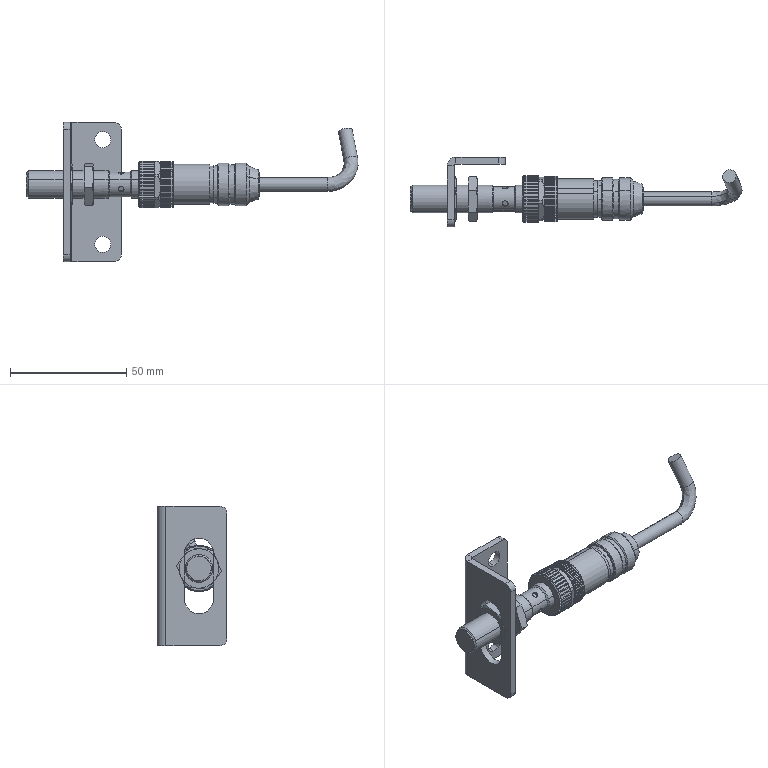Part | SolidWorks | 3 solids | 685 faces | box 143.072 x 30 x 60 mm | volume 24303 mm3 | plane 364 | cylinder 199 | cone 120 | spline 2 | commonest cylinder face diameters 19.5 x50 20 x38 2.5 x12 12 x10 1 x8 1.1 x8